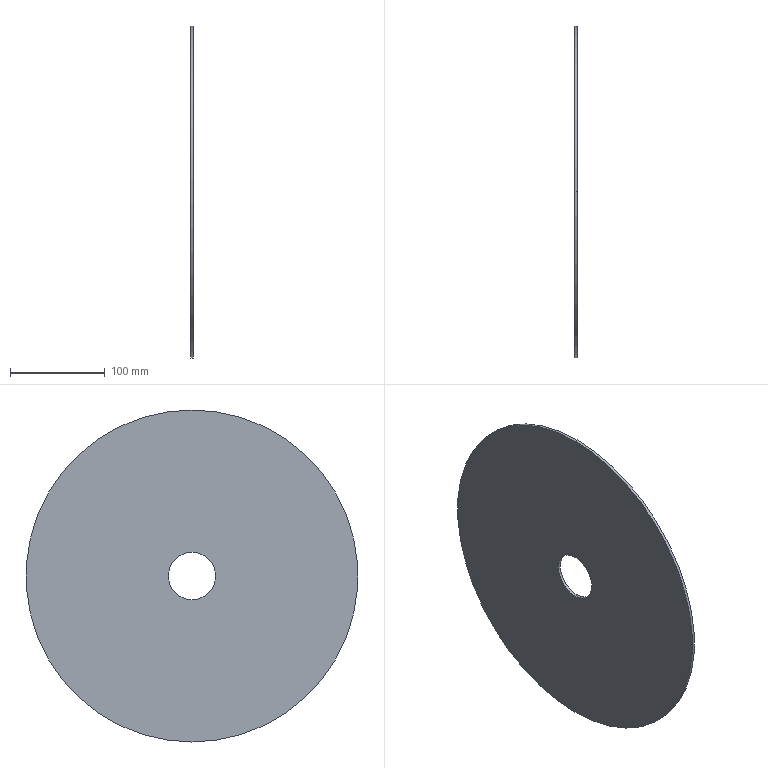Part | SolidWorks | features ICE 4, Chamfer 1, Extrusion 1, RevCut 1 | 1 solid | 6 faces | box 3 x 350 x 350 mm | volume 282743 mm3 | cylinder 4 | plane 2 | commonest cylinder face diameters 50 x2 350 x2
STEP:
#1=CARTESIAN_POINT('',(1.3,0.,175.));
#2=VERTEX_POINT('',#1);
#3=CARTESIAN_POINT('',(1.3,0.,-175.));
#4=VERTEX_POINT('',#3);
#5=CARTESIAN_POINT('',(1.3,0.,0.));
#6=DIRECTION('',(-1.,0.,0.));
#7=DIRECTION('',(0.,0.,1.));
#8=AXIS2_PLACEMENT_3D('',#5,#6,#7);
#9=CIRCLE('',#8,175.);
#10=EDGE_CURVE('',#2,#4,#9,.T.);
#11=ORIENTED_EDGE('',*,*,#10,.T.);
#12=CARTESIAN_POINT('',(-1.7,0.,-175.));
#13=VERTEX_POINT('',#12);
#14=CARTESIAN_POINT('',(8.,0.,-175.));
#15=DIRECTION('',(-1.,0.,0.));
#16=VECTOR('',#15,1000.);
#17=LINE('',#14,#16);
#18=EDGE_CURVE('',#4,#13,#17,.T.);
#19=ORIENTED_EDGE('',*,*,#18,.T.);
#20=CARTESIAN_POINT('',(-1.7,0.,175.));
#21=VERTEX_POINT('',#20);
#22=CARTESIAN_POINT('',(-1.7,0.,0.));
#23=DIRECTION('',(1.,0.,0.));
#24=DIRECTION('',(0.,0.,-1.));
#25=AXIS2_PLACEMENT_3D('',#22,#23,#24);
#26=CIRCLE('',#25,175.);
#27=EDGE_CURVE('',#13,#21,#26,.T.);
#28=ORIENTED_EDGE('',*,*,#27,.T.);
#29=CARTESIAN_POINT('',(8.,0.,175.));
#30=DIRECTION('',(-1.,0.,0.));
#31=VECTOR('',#30,1000.);
#32=LINE('',#29,#31);
#33=EDGE_CURVE('',#2,#21,#32,.T.);
#34=ORIENTED_EDGE('',*,*,#33,.F.);
#35=EDGE_LOOP('',(#11,#19,#28,#34));
#36=FACE_OUTER_BOUND('',#35,.T.);
#37=CARTESIAN_POINT('',(8.,0.,0.));
#38=DIRECTION('',(-1.,0.,0.));
#39=DIRECTION('',(0.,0.,1.));
#40=AXIS2_PLACEMENT_3D('',#37,#38,#39);
#41=CYLINDRICAL_SURFACE('',#40,175.);
#42=ADVANCED_FACE('',(#36),#41,.T.);
#43=CARTESIAN_POINT('',(-1.7,0.,25.));
#44=VERTEX_POINT('',#43);
#45=CARTESIAN_POINT('',(-1.7,0.,-25.));
#46=VERTEX_POINT('',#45);
#47=CARTESIAN_POINT('',(-1.7,0.,0.));
#48=DIRECTION('',(1.,0.,0.));
#49=DIRECTION('',(0.,0.,-1.));
#50=AXIS2_PLACEMENT_3D('',#47,#48,#49);
#51=CIRCLE('',#50,25.);
#52=EDGE_CURVE('',#44,#46,#51,.T.);
#53=ORIENTED_EDGE('',*,*,#52,.F.);
#54=CARTESIAN_POINT('',(1.3,0.,25.));
#55=VERTEX_POINT('',#54);
#56=CARTESIAN_POINT('',(-1.7,0.,25.));
#57=DIRECTION('',(1.,0.,0.));
#58=VECTOR('',#57,1000.);
#59=LINE('',#56,#58);
#60=EDGE_CURVE('',#44,#55,#59,.T.);
#61=ORIENTED_EDGE('',*,*,#60,.T.);
#62=CARTESIAN_POINT('',(1.3,0.,-25.));
#63=VERTEX_POINT('',#62);
#64=CARTESIAN_POINT('',(1.3,0.,0.));
#65=DIRECTION('',(1.,0.,0.));
#66=DIRECTION('',(0.,0.,-1.));
#67=AXIS2_PLACEMENT_3D('',#64,#65,#66);
#68=CIRCLE('',#67,25.);
#69=EDGE_CURVE('',#55,#63,#68,.T.);
#70=ORIENTED_EDGE('',*,*,#69,.T.);
#71=CARTESIAN_POINT('',(-1.7,0.,-25.));
#72=DIRECTION('',(1.,0.,0.));
#73=VECTOR('',#72,1000.);
#74=LINE('',#71,#73);
#75=EDGE_CURVE('',#46,#63,#74,.T.);
#76=ORIENTED_EDGE('',*,*,#75,.F.);
#77=EDGE_LOOP('',(#53,#61,#70,#76));
#78=FACE_OUTER_BOUND('',#77,.T.);
#79=CARTESIAN_POINT('',(-1.7,0.,0.));
#80=DIRECTION('',(1.,0.,0.));
#81=DIRECTION('',(0.,0.,-1.));
#82=AXIS2_PLACEMENT_3D('',#79,#80,#81);
#83=CYLINDRICAL_SURFACE('',#82,25.);
#84=ADVANCED_FACE('',(#78),#83,.F.);
#85=CARTESIAN_POINT('',(-1.7,0.,0.));
#86=DIRECTION('',(1.,0.,0.));
#87=DIRECTION('',(0.,0.,-1.));
#88=AXIS2_PLACEMENT_3D('',#85,#86,#87);
#89=CIRCLE('',#88,25.);
#90=EDGE_CURVE('',#46,#44,#89,.T.);
#91=ORIENTED_EDGE('',*,*,#90,.T.);
#92=ORIENTED_EDGE('',*,*,#52,.T.);
#93=EDGE_LOOP('',(#91,#92));
#94=FACE_BOUND('',#93,.T.);
#95=CARTESIAN_POINT('',(-1.7,0.,0.));
#96=DIRECTION('',(1.,0.,0.));
#97=DIRECTION('',(0.,0.,-1.));
#98=AXIS2_PLACEMENT_3D('',#95,#96,#97);
#99=CIRCLE('',#98,175.);
#100=EDGE_CURVE('',#21,#13,#99,.T.);
#101=ORIENTED_EDGE('',*,*,#100,.F.);
#102=ORIENTED_EDGE('',*,*,#27,.F.);
#103=EDGE_LOOP('',(#101,#102));
#104=FACE_OUTER_BOUND('',#103,.T.);
#105=CARTESIAN_POINT('',(-1.7,-4.515,-191.575));
#106=DIRECTION('',(1.,0.,0.));
#107=DIRECTION('',(0.,0.,-1.));
#108=AXIS2_PLACEMENT_3D('',#105,#106,#107);
#109=PLANE('',#108);
#110=ADVANCED_FACE('',(#94,#104),#109,.F.);
#111=CARTESIAN_POINT('',(1.3,0.,0.));
#112=DIRECTION('',(1.,0.,0.));
#113=DIRECTION('',(0.,0.,-1.));
#114=AXIS2_PLACEMENT_3D('',#111,#112,#113);
#115=CIRCLE('',#114,25.);
#116=EDGE_CURVE('',#63,#55,#115,.T.);
#117=ORIENTED_EDGE('',*,*,#116,.F.);
#118=ORIENTED_EDGE('',*,*,#69,.F.);
#119=EDGE_LOOP('',(#117,#118));
#120=FACE_BOUND('',#119,.T.);
#121=ORIENTED_EDGE('',*,*,#10,.F.);
#122=CARTESIAN_POINT('',(1.3,0.,0.));
#123=DIRECTION('',(-1.,0.,0.));
#124=DIRECTION('',(0.,0.,1.));
#125=AXIS2_PLACEMENT_3D('',#122,#123,#124);
#126=CIRCLE('',#125,175.);
#127=EDGE_CURVE('',#4,#2,#126,.T.);
#128=ORIENTED_EDGE('',*,*,#127,.F.);
#129=EDGE_LOOP('',(#121,#128));
#130=FACE_OUTER_BOUND('',#129,.T.);
#131=CARTESIAN_POINT('',(1.3,-63.494,-180.804));
#132=DIRECTION('',(-1.,0.,0.));
#133=DIRECTION('',(0.,0.,1.));
#134=AXIS2_PLACEMENT_3D('',#131,#132,#133);
#135=PLANE('',#134);
#136=ADVANCED_FACE('',(#120,#130),#135,.F.);
#137=ORIENTED_EDGE('',*,*,#60,.F.);
#138=ORIENTED_EDGE('',*,*,#90,.F.);
#139=ORIENTED_EDGE('',*,*,#75,.T.);
#140=ORIENTED_EDGE('',*,*,#116,.T.);
#141=EDGE_LOOP('',(#137,#138,#139,#140));
#142=FACE_OUTER_BOUND('',#141,.T.);
#143=CARTESIAN_POINT('',(-1.7,0.,0.));
#144=DIRECTION('',(1.,0.,0.));
#145=DIRECTION('',(0.,0.,-1.));
#146=AXIS2_PLACEMENT_3D('',#143,#144,#145);
#147=CYLINDRICAL_SURFACE('',#146,25.);
#148=ADVANCED_FACE('',(#142),#147,.F.);
#149=ORIENTED_EDGE('',*,*,#18,.F.);
#150=ORIENTED_EDGE('',*,*,#127,.T.);
#151=ORIENTED_EDGE('',*,*,#33,.T.);
#152=ORIENTED_EDGE('',*,*,#100,.T.);
#153=EDGE_LOOP('',(#149,#150,#151,#152));
#154=FACE_OUTER_BOUND('',#153,.T.);
#155=CARTESIAN_POINT('',(8.,0.,0.));
#156=DIRECTION('',(-1.,0.,0.));
#157=DIRECTION('',(0.,0.,1.));
#158=AXIS2_PLACEMENT_3D('',#155,#156,#157);
#159=CYLINDRICAL_SURFACE('',#158,175.);
#160=ADVANCED_FACE('',(#154),#159,.T.);
#161=CLOSED_SHELL('',(#42,#84,#110,#136,#148,#160));
#162=MANIFOLD_SOLID_BREP('',#161);
#163=CARTESIAN_POINT('',(0.,0.,0.));
#164=DIRECTION('',(0.,0.,1.));
#165=DIRECTION('',(1.,0.,0.));
#166=AXIS2_PLACEMENT_3D('',#163,#164,#165);
#167=(LENGTH_UNIT()NAMED_UNIT(*)SI_UNIT(.MILLI.,.METRE.));
#168=UNCERTAINTY_MEASURE_WITH_UNIT(LENGTH_MEASURE(0.00001),#167,'','');
#169=(NAMED_UNIT(*)PLANE_ANGLE_UNIT()SI_UNIT($,.RADIAN.));
#170=(NAMED_UNIT(*)SI_UNIT($,.STERADIAN.)SOLID_ANGLE_UNIT());
#171=(GEOMETRIC_REPRESENTATION_CONTEXT(3)GLOBAL_UNCERTAINTY_ASSIGNED_CONTEXT((#168))GLOBAL_UNIT_ASSIGNED_CONTEXT((#167,#169,#170))REPRESENTATION_CONTEXT('',''));
#172=ADVANCED_BREP_SHAPE_REPRESENTATION('',(#162,#166),#171);